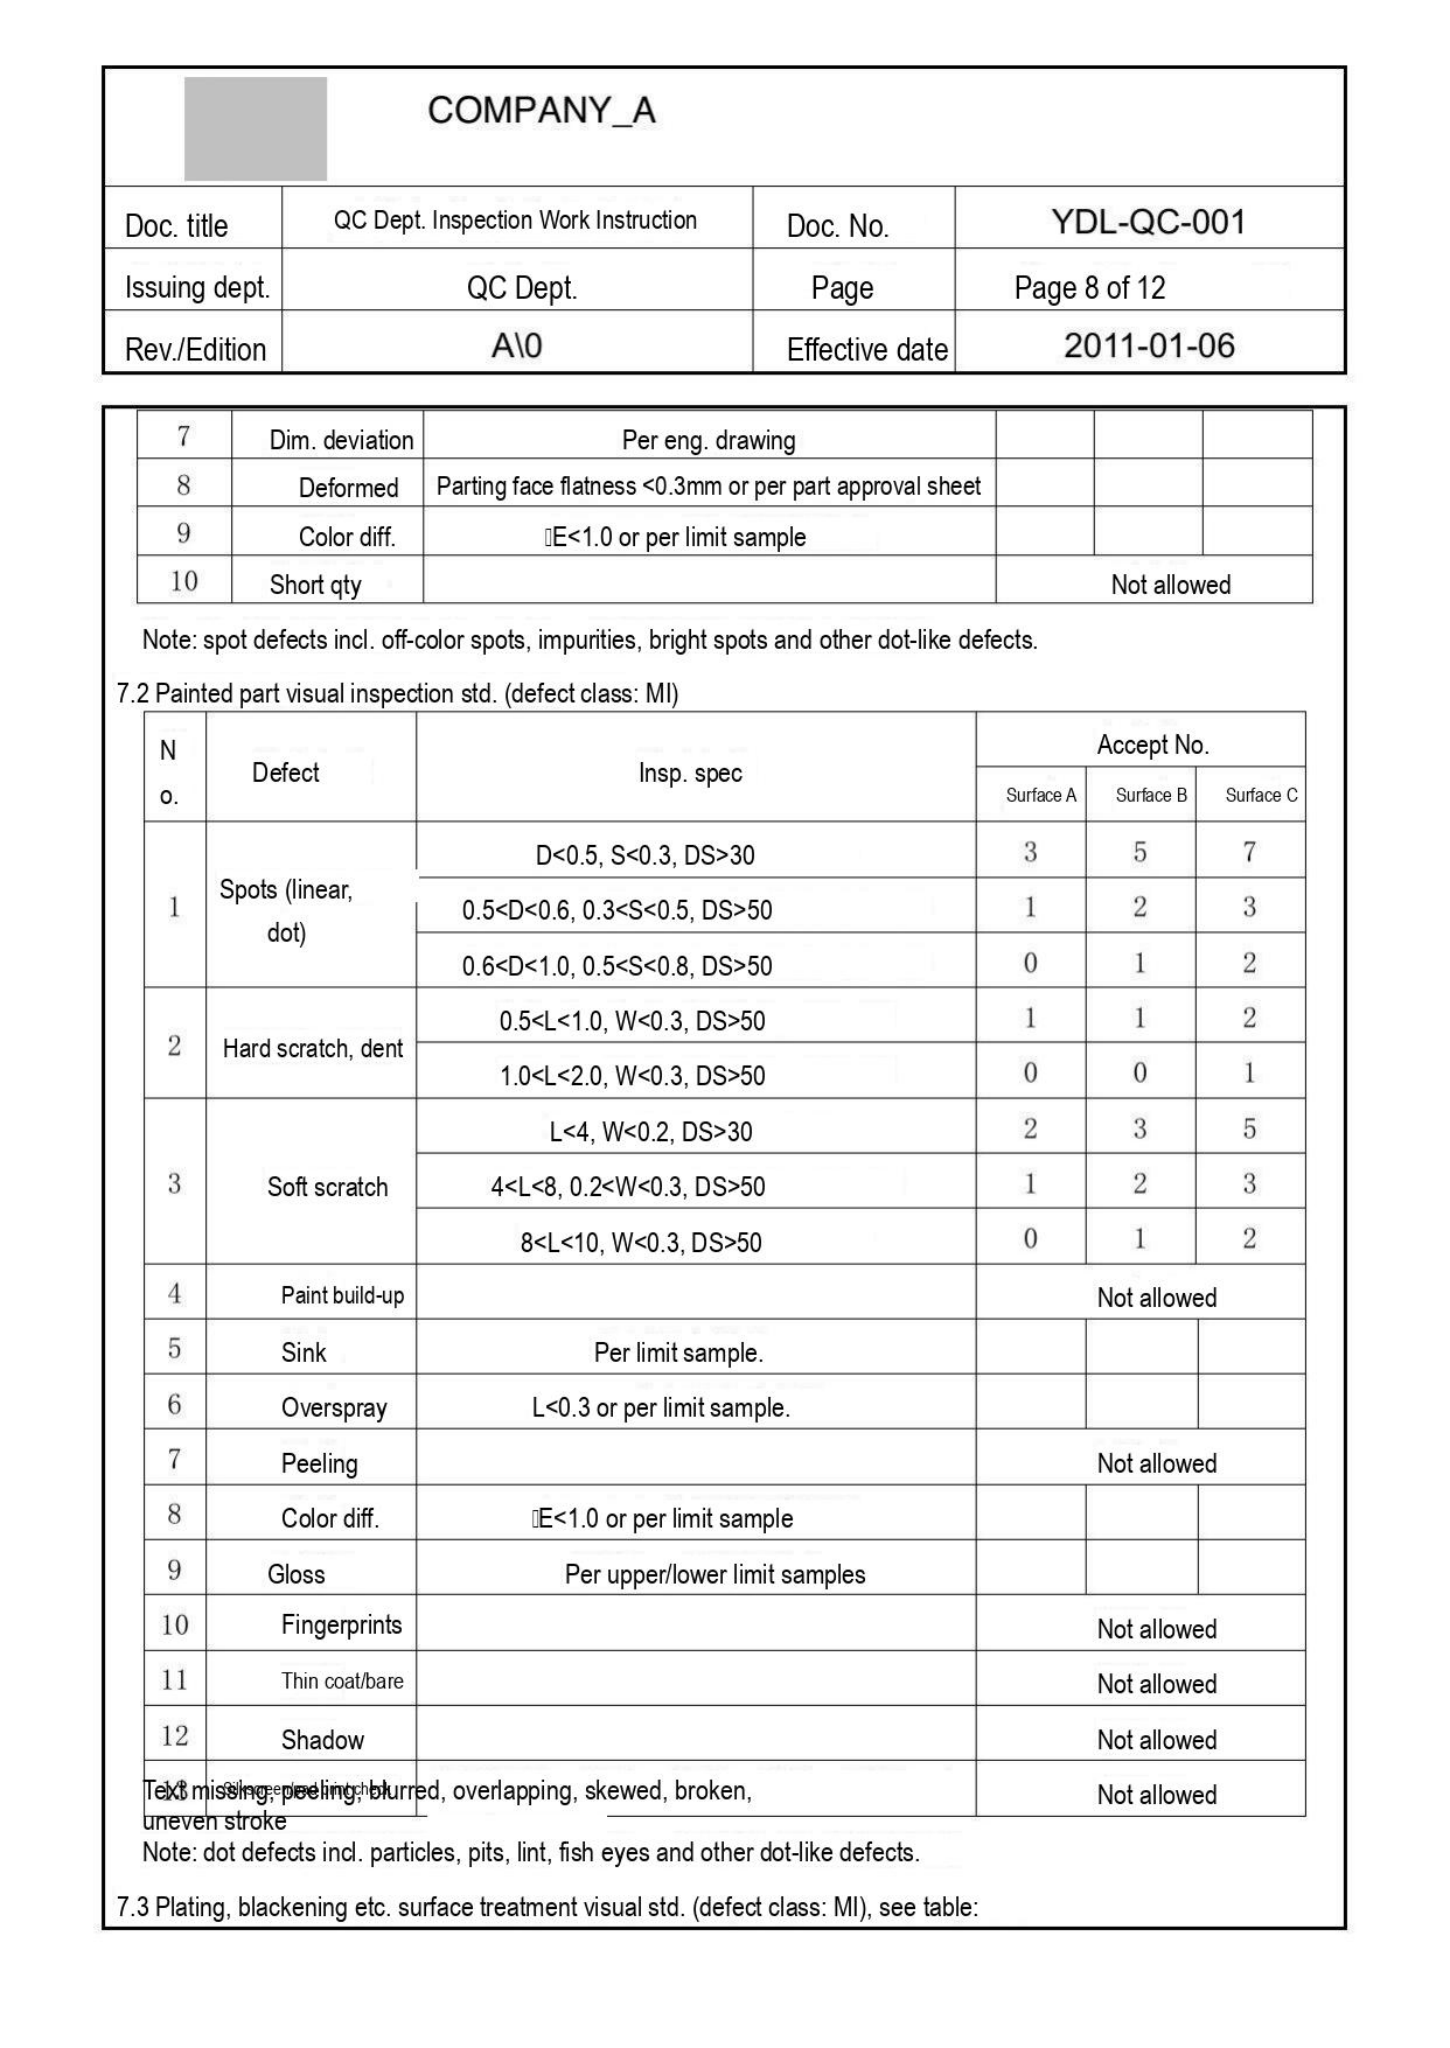| COMPANY_A | | | |
|---|---|---|---|
| Doc. title | QC Dept. Inspection Work Instruction | Doc. No. | YDL-QC-001 |
| Issuing dept. | QC Dept. | Page | Page 8 of 12 |
| Rev./Edition | A\0 | Effective date | 2011-01-06 |

| | | | | | |
|---|---|---|---|---|---|
| 7 | Dim. deviation | Per eng. drawing | | | |
| 8 | Deformed | Parting face flatness <0.3mm or per part approval sheet | | | |
| 9 | Color diff. | E<1.0 or per limit sample | | | |
| 10 | Short qty | | Not allowed | | |

Note: spot defects incl. off-color spots, impurities, bright spots and other dot-like defects.

7.2 Painted part visual inspection std. (defect class: MI)

| No. | Defect | Insp. spec | Accept No. Surface A | Accept No. Surface B | Accept No. Surface C |
|---|---|---|---|---|---|
| 1 | Spots (linear, dot) | D<0.5, S<0.3, DS>30 | 3 | 5 | 7 |
| | | 0.5<D<0.6, 0.3<S<0.5, DS>50 | 1 | 2 | 3 |
| | | 0.6<D<1.0, 0.5<S<0.8, DS>50 | 0 | 1 | 2 |
| 2 | Hard scratch, dent | 0.5<L<1.0, W<0.3, DS>50 | 1 | 1 | 2 |
| | | 1.0<L<2.0, W<0.3, DS>50 | 0 | 0 | 1 |
| 3 | Soft scratch | L<4, W<0.2, DS>30 | 2 | 3 | 5 |
| | | 4<L<8, 0.2<W<0.3, DS>50 | 1 | 2 | 3 |
| | | 8<L<10, W<0.3, DS>50 | 0 | 1 | 2 |
| 4 | Paint build-up | | Not allowed | | |
| 5 | Sink | Per limit sample. | | | |
| 6 | Overspray | L<0.3 or per limit sample. | | | |
| 7 | Peeling | | Not allowed | | |
| 8 | Color diff. | E<1.0 or per limit sample | | | |
| 9 | Gloss | Per upper/lower limit samples | | | |
| 10 | Fingerprints | | Not allowed | | |
| 11 | Thin coat/bare | | Not allowed | | |
| 12 | Shadow | | Not allowed | | |
| 13 | | Text missing, peeling, blurred, overlapping, skewed, broken, uneven stroke | Not allowed | | |

Note: dot defects incl. particles, pits, lint, fish eyes and other dot-like defects.

7.3 Plating, blackening etc. surface treatment visual std. (defect class: MI), see table:
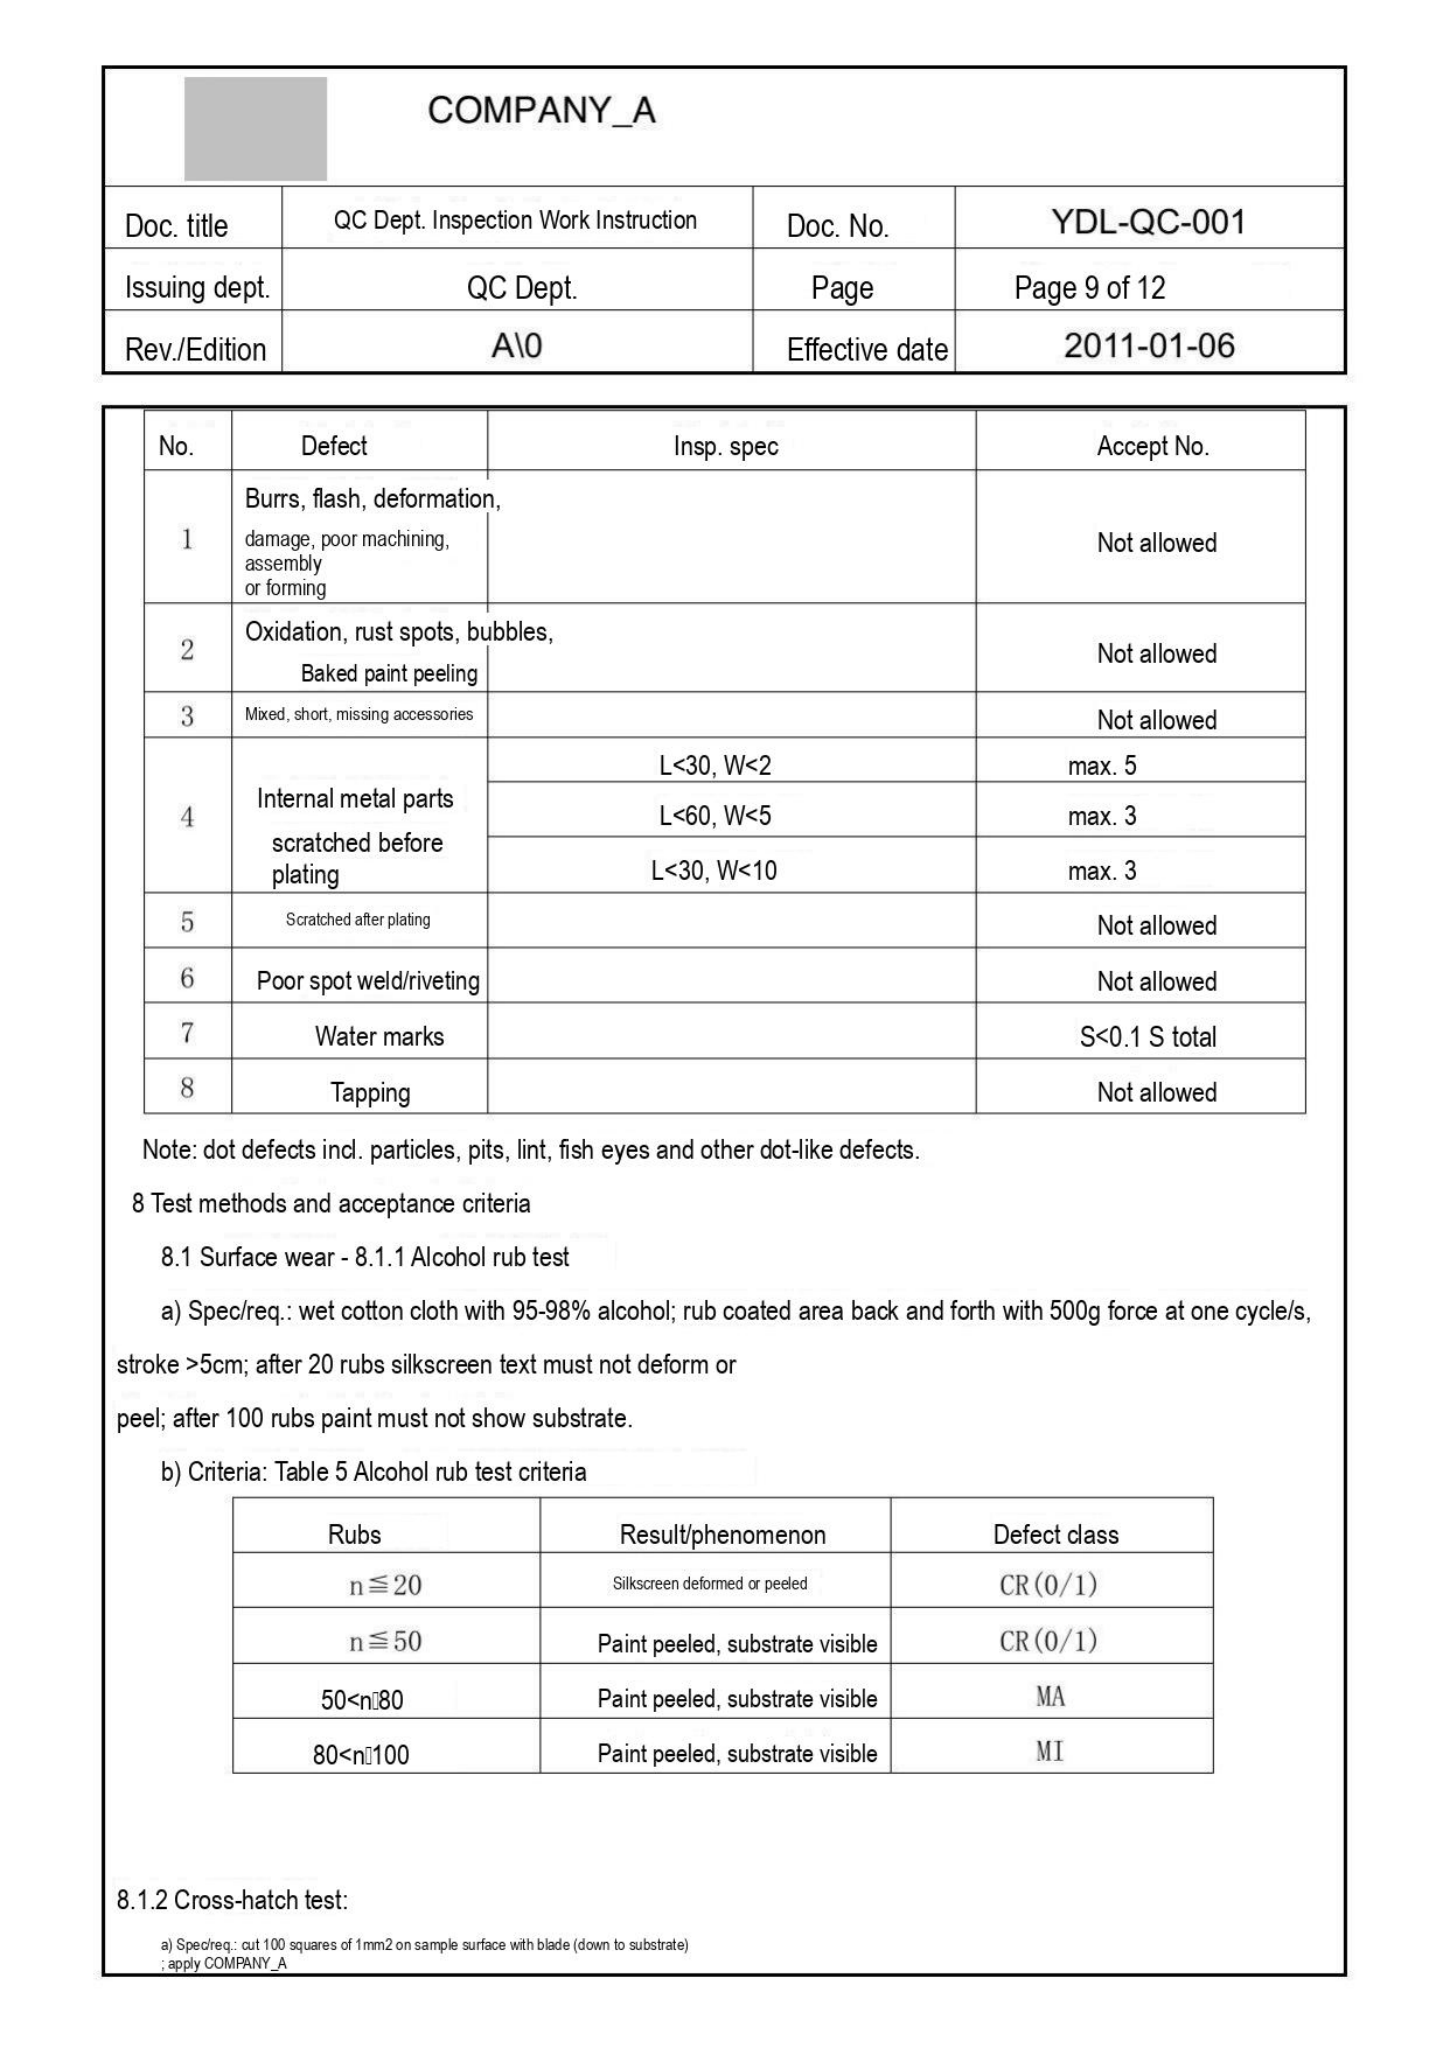COMPANY_A

| Doc. title | QC Dept. Inspection Work Instruction | Doc. No. | YDL-QC-001 |
|---|---|---|---|
| Issuing dept. | QC Dept. | Page | Page 9 of 12 |
| Rev./Edition | A\0 | Effective date | 2011-01-06 |

| No. | Defect | Insp. spec | Accept No. |
|---|---|---|---|
| 1 | Burrs, flash, deformation, damage, poor machining, assembly or forming | | Not allowed |
| 2 | Oxidation, rust spots, bubbles, Baked paint peeling | | Not allowed |
| 3 | Mixed, short, missing accessories | | Not allowed |
| 4 | Internal metal parts scratched before plating | L<30, W<2 | max. 5 |
| | | L<60, W<5 | max. 3 |
| | | L<30, W<10 | max. 3 |
| 5 | Scratched after plating | | Not allowed |
| 6 | Poor spot weld/riveting | | Not allowed |
| 7 | Water marks | | S<0.1 S total |
| 8 | Tapping | | Not allowed |

Note: dot defects incl. particles, pits, lint, fish eyes and other dot-like defects.

8 Test methods and acceptance criteria

8.1 Surface wear - 8.1.1 Alcohol rub test

a) Spec/req.: wet cotton cloth with 95-98% alcohol; rub coated area back and forth with 500g force at one cycle/s, stroke >5cm; after 20 rubs silkscreen text must not deform or peel; after 100 rubs paint must not show substrate.

b) Criteria: Table 5 Alcohol rub test criteria

| Rubs | Result/phenomenon | Defect class |
|---|---|---|
| n≦20 | Silkscreen deformed or peeled | CR(0/1) |
| n≦50 | Paint peeled, substrate visible | CR(0/1) |
| 50<n80 | Paint peeled, substrate visible | MA |
| 80<n100 | Paint peeled, substrate visible | MI |

8.1.2 Cross-hatch test:

a) Spec/req.: cut 100 squares of 1mm2 on sample surface with blade (down to substrate) ; apply COMPANY_A
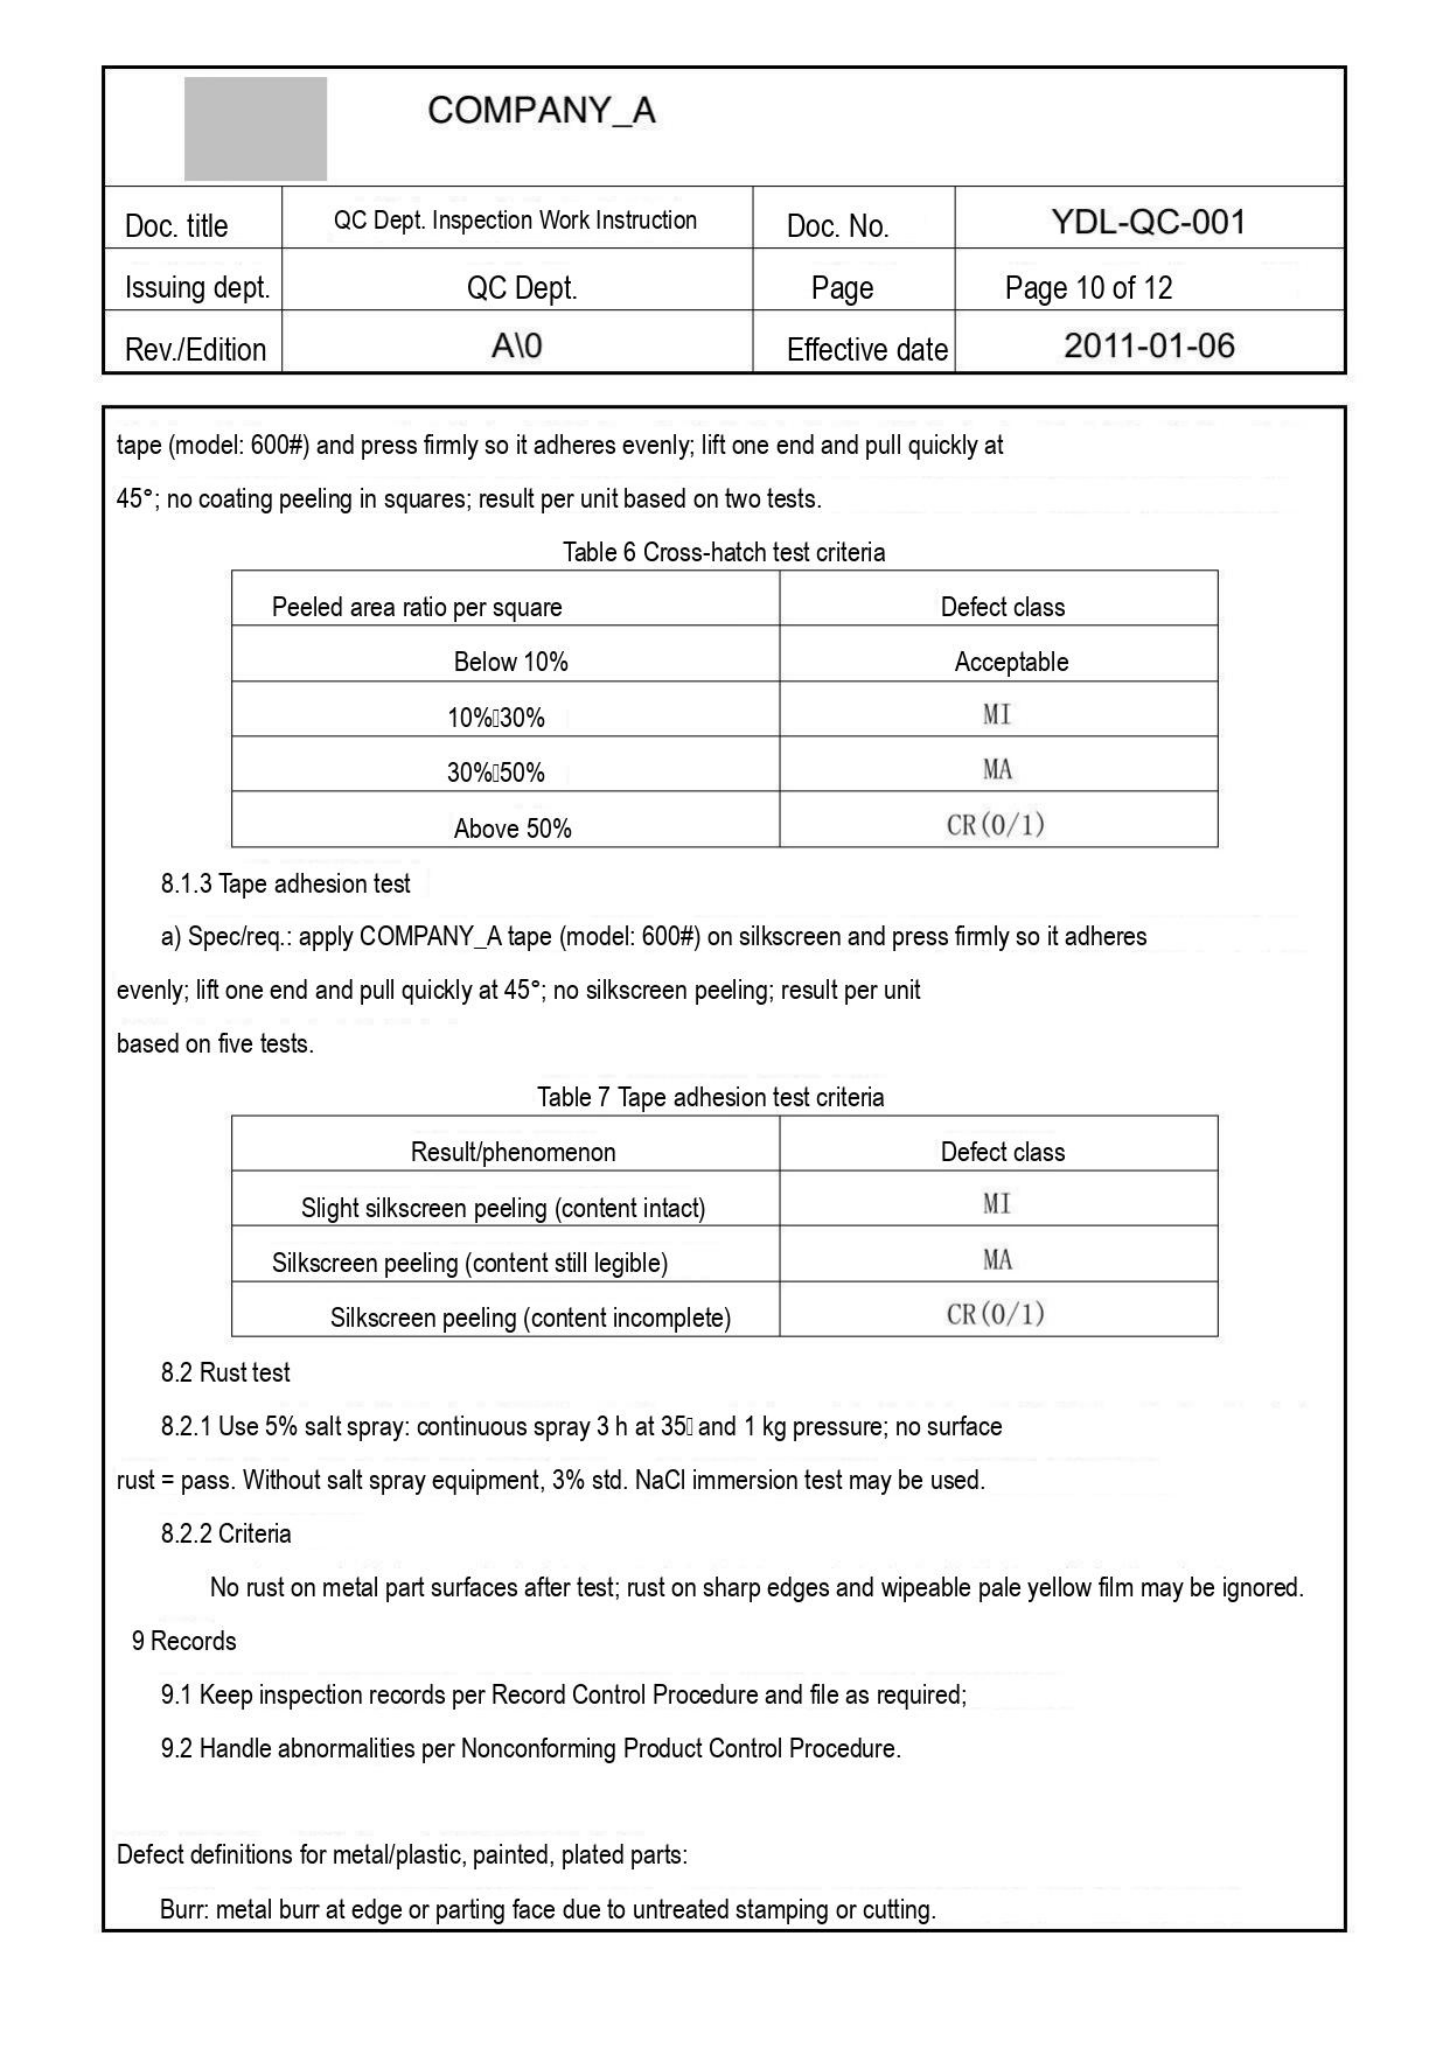COMPANY_A

| Doc. title | QC Dept. Inspection Work Instruction | Doc. No. | YDL-QC-001 |
|---|---|---|---|
| Issuing dept. | QC Dept. | Page | Page 10 of 12 |
| Rev./Edition | A\0 | Effective date | 2011-01-06 |

tape (model: 600#) and press firmly so it adheres evenly; lift one end and pull quickly at 45°; no coating peeling in squares; result per unit based on two tests.

Table 6 Cross-hatch test criteria

| Peeled area ratio per square | Defect class |
|---|---|
| Below 10% | Acceptable |
| 10%30% | MI |
| 30%50% | MA |
| Above 50% | CR(0/1) |

8.1.3 Tape adhesion test

a) Spec/req.: apply COMPANY_A tape (model: 600#) on silkscreen and press firmly so it adheres evenly; lift one end and pull quickly at 45°; no silkscreen peeling; result per unit based on five tests.

Table 7 Tape adhesion test criteria

| Result/phenomenon | Defect class |
|---|---|
| Slight silkscreen peeling (content intact) | MI |
| Silkscreen peeling (content still legible) | MA |
| Silkscreen peeling (content incomplete) | CR(0/1) |

8.2 Rust test

8.2.1 Use 5% salt spray: continuous spray 3 h at 35 and 1 kg pressure; no surface rust = pass. Without salt spray equipment, 3% std. NaCl immersion test may be used.

8.2.2 Criteria

No rust on metal part surfaces after test; rust on sharp edges and wipeable pale yellow film may be ignored.

9 Records

9.1 Keep inspection records per Record Control Procedure and file as required;

9.2 Handle abnormalities per Nonconforming Product Control Procedure.

Defect definitions for metal/plastic, painted, plated parts:

Burr: metal burr at edge or parting face due to untreated stamping or cutting.
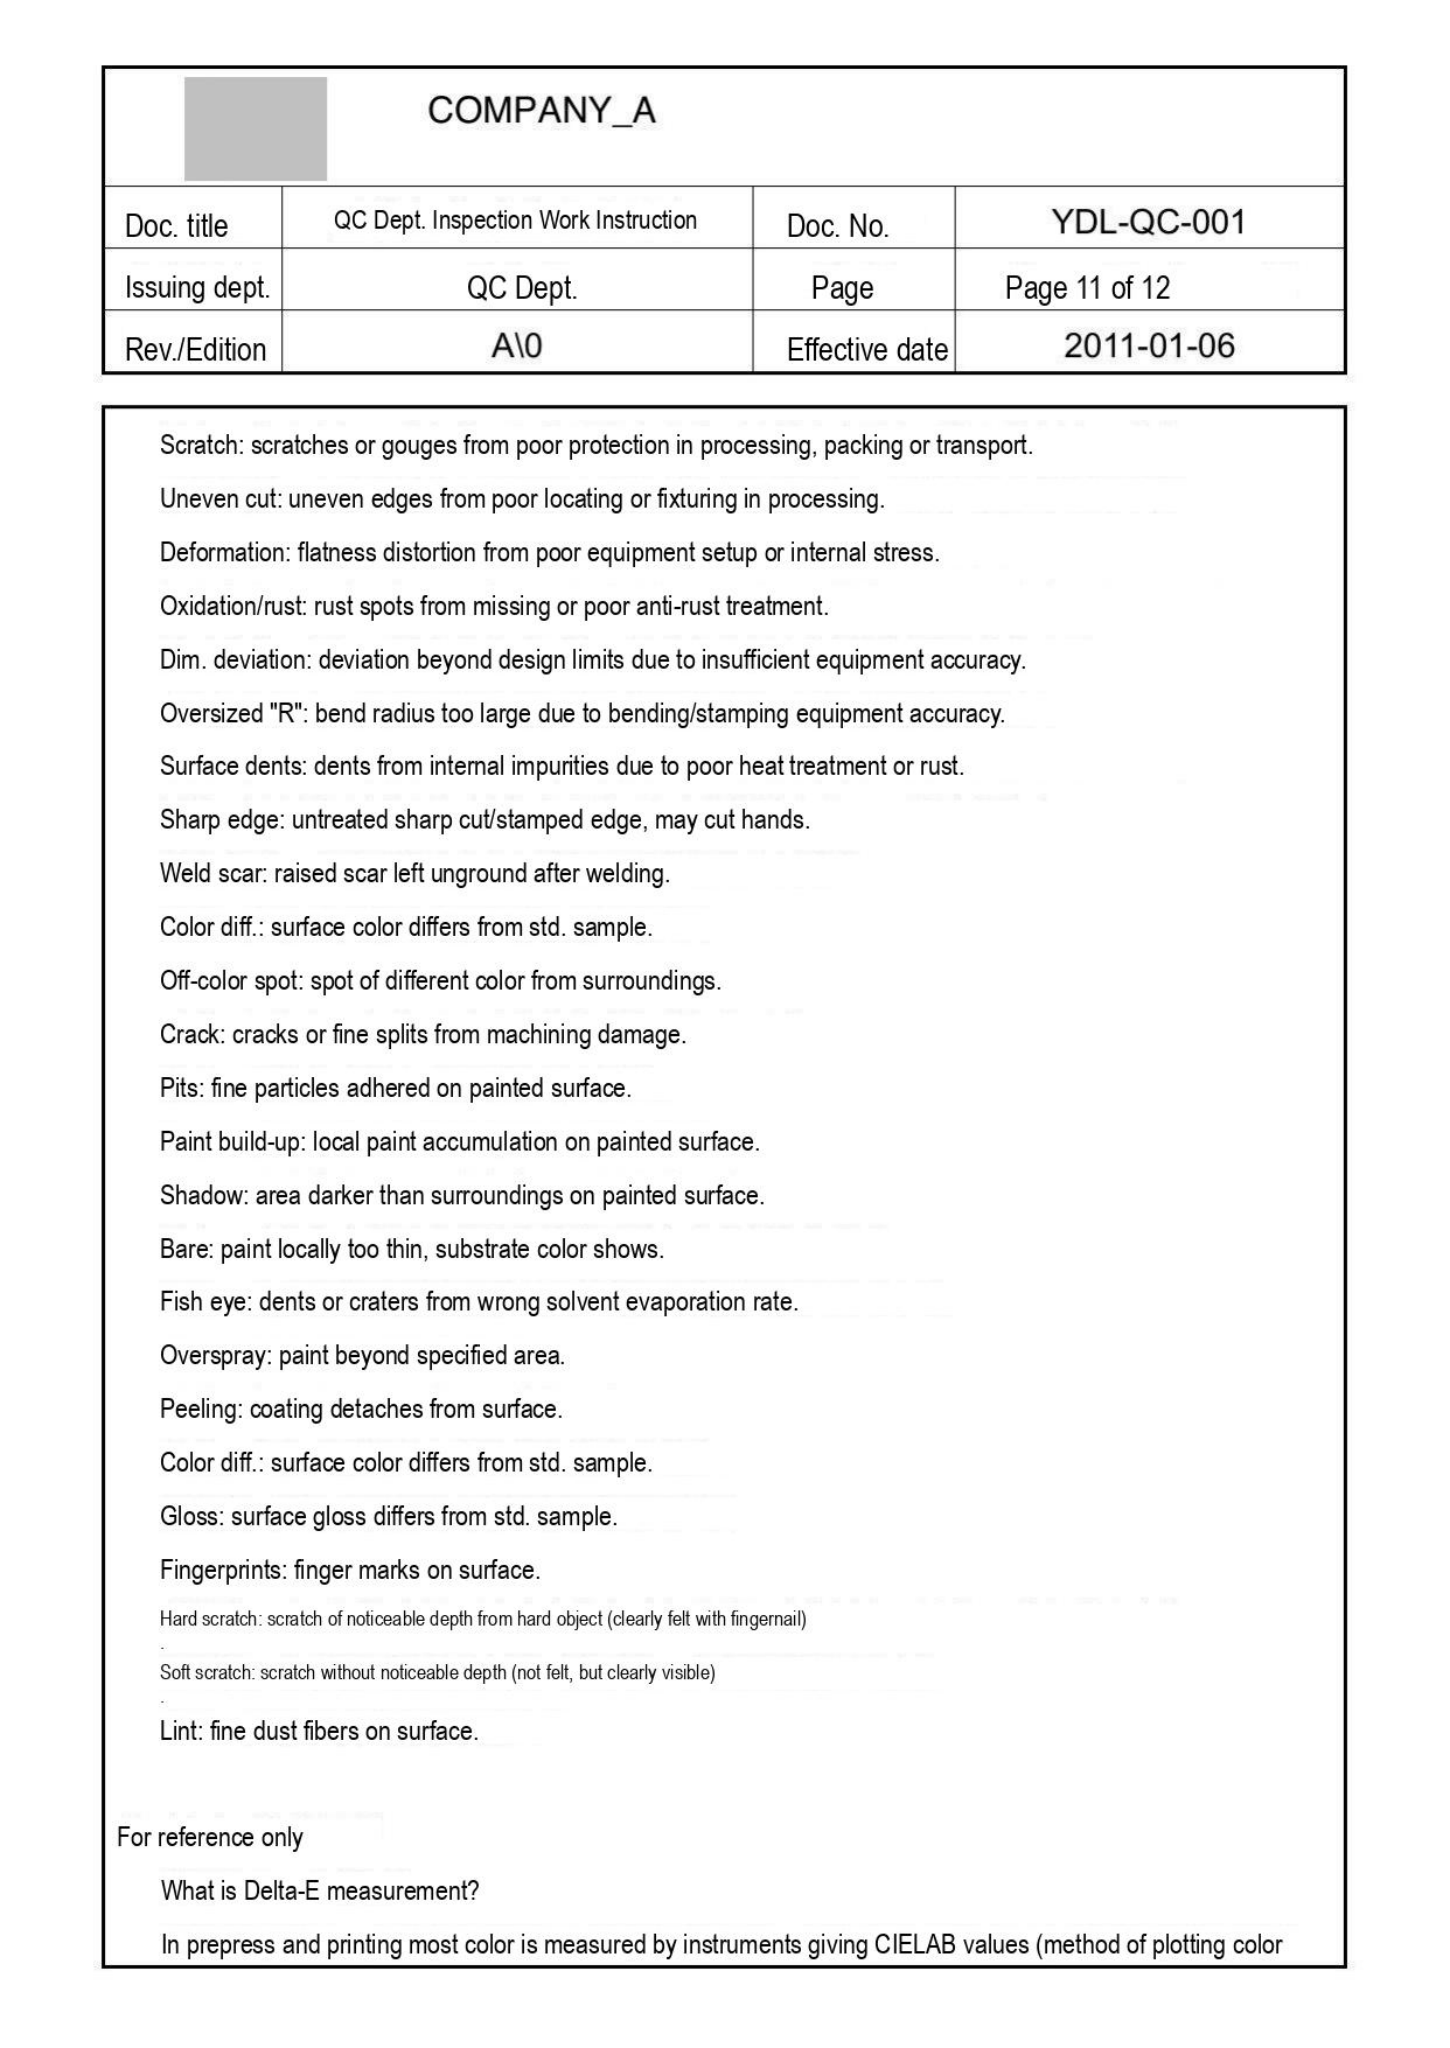COMPANY_A

| Doc. title | QC Dept. Inspection Work Instruction | Doc. No. | YDL-QC-001 |
|---|---|---|---|
| Issuing dept. | QC Dept. | Page | Page 11 of 12 |
| Rev./Edition | A\0 | Effective date | 2011-01-06 |

Scratch: scratches or gouges from poor protection in processing, packing or transport.

Uneven cut: uneven edges from poor locating or fixturing in processing.

Deformation: flatness distortion from poor equipment setup or internal stress.

Oxidation/rust: rust spots from missing or poor anti-rust treatment.

Dim. deviation: deviation beyond design limits due to insufficient equipment accuracy.

Oversized "R": bend radius too large due to bending/stamping equipment accuracy.

Surface dents: dents from internal impurities due to poor heat treatment or rust.

Sharp edge: untreated sharp cut/stamped edge, may cut hands.

Weld scar: raised scar left unground after welding.

Color diff.: surface color differs from std. sample.

Off-color spot: spot of different color from surroundings.

Crack: cracks or fine splits from machining damage.

Pits: fine particles adhered on painted surface.

Paint build-up: local paint accumulation on painted surface.

Shadow: area darker than surroundings on painted surface.

Bare: paint locally too thin, substrate color shows.

Fish eye: dents or craters from wrong solvent evaporation rate.

Overspray: paint beyond specified area.

Peeling: coating detaches from surface.

Color diff.: surface color differs from std. sample.

Gloss: surface gloss differs from std. sample.

Fingerprints: finger marks on surface.

Hard scratch: scratch of noticeable depth from hard object (clearly felt with fingernail)

Soft scratch: scratch without noticeable depth (not felt, but clearly visible)

Lint: fine dust fibers on surface.

For reference only

What is Delta-E measurement?

In prepress and printing most color is measured by instruments giving CIELAB values (method of plotting color
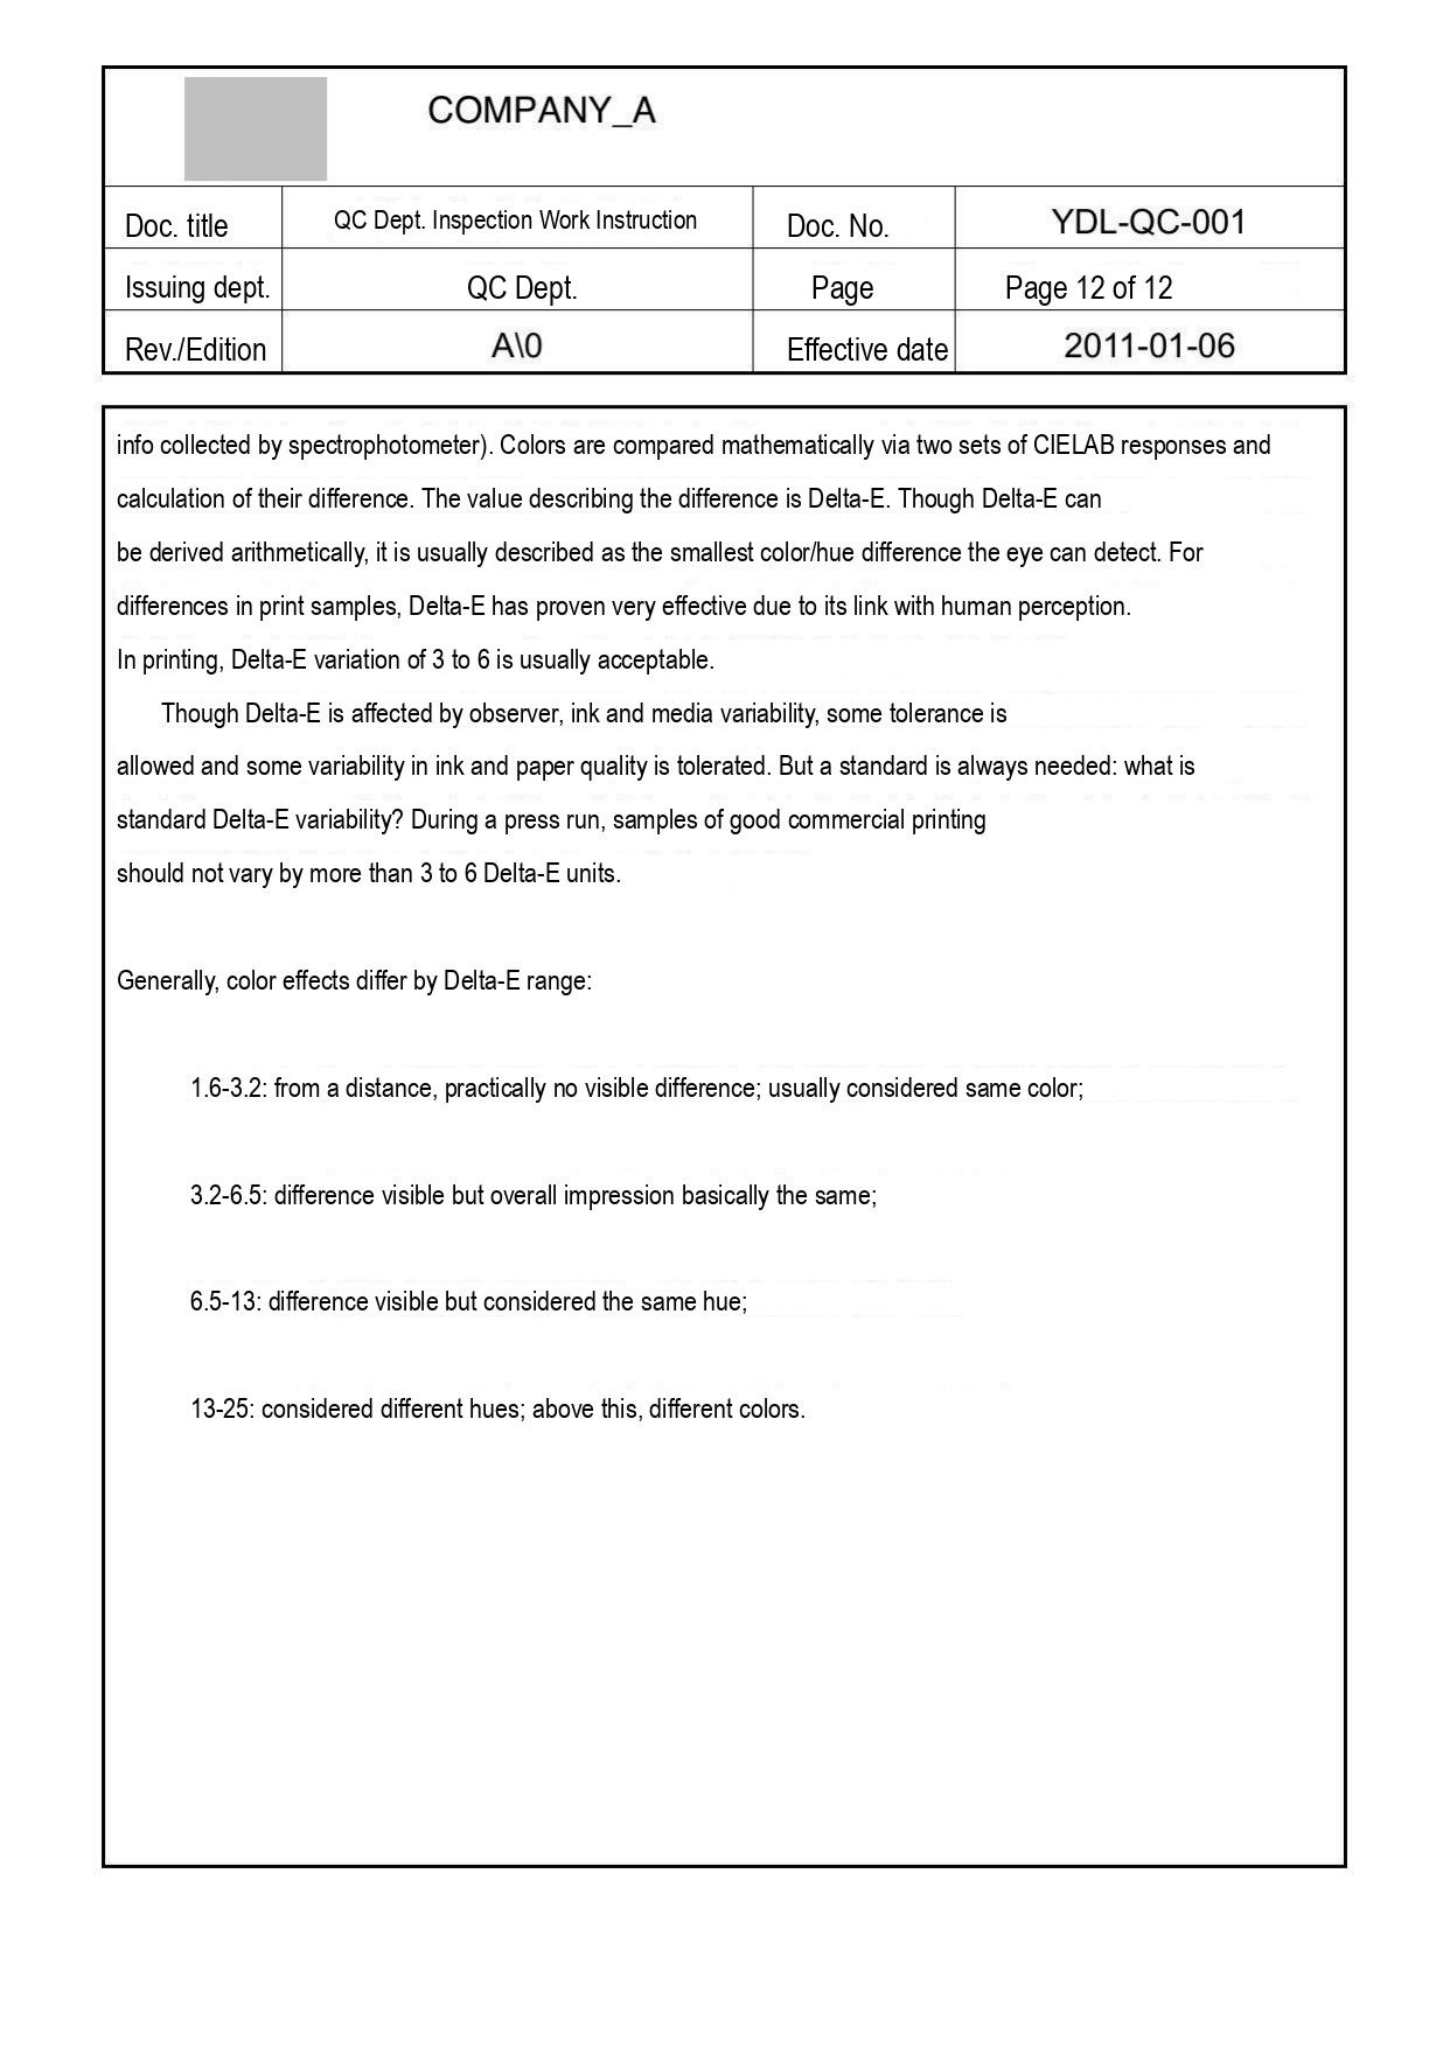COMPANY_A

| Doc. title | QC Dept. Inspection Work Instruction | Doc. No. | YDL-QC-001 |
|---|---|---|---|
| Issuing dept. | QC Dept. | Page | Page 12 of 12 |
| Rev./Edition | A\0 | Effective date | 2011-01-06 |

info collected by spectrophotometer). Colors are compared mathematically via two sets of CIELAB responses and calculation of their difference. The value describing the difference is Delta-E. Though Delta-E can be derived arithmetically, it is usually described as the smallest color/hue difference the eye can detect. For differences in print samples, Delta-E has proven very effective due to its link with human perception.
In printing, Delta-E variation of 3 to 6 is usually acceptable.

Though Delta-E is affected by observer, ink and media variability, some tolerance is allowed and some variability in ink and paper quality is tolerated. But a standard is always needed: what is standard Delta-E variability? During a press run, samples of good commercial printing should not vary by more than 3 to 6 Delta-E units.

Generally, color effects differ by Delta-E range:

1.6-3.2: from a distance, practically no visible difference; usually considered same color;

3.2-6.5: difference visible but overall impression basically the same;

6.5-13: difference visible but considered the same hue;

13-25: considered different hues; above this, different colors.